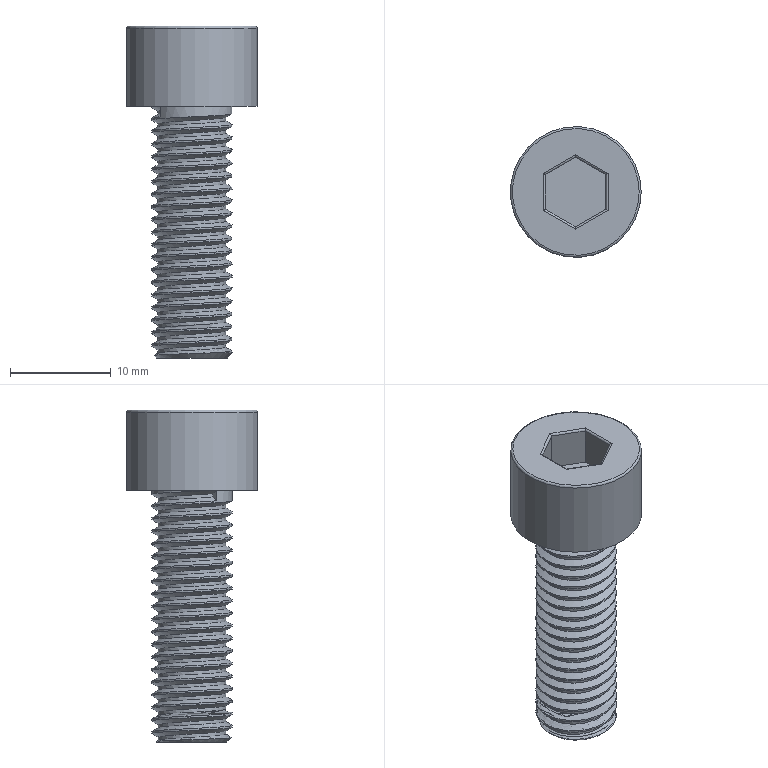Part | STEP file | Tube feed_id1130_x_t | 1 solid | 26 faces | box 13 x 13 x 33 mm | volume 1997 mm3 | plane 12 | cylinder 9 | spline 3 | torus 1 | cone 1 | commonest cylinder face diameters 0.4 x6 6.75 x1 8 x1 13 x1